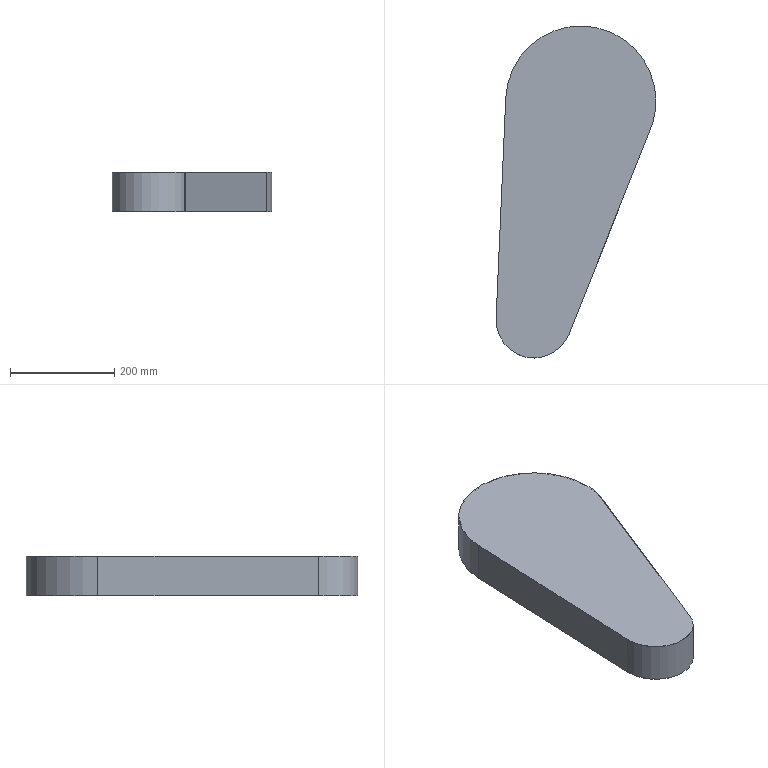Part | SolidWorks | features BaseBody 1 | 1 solid | 13 faces | box 306.5 x 636.5 x 76.6 mm | volume 401718 mm3 | plane 7 | cylinder 6 | commonest cylinder face diameters 141.8 x2 288 x2 145 x1 284.8 x1
STEP:
#1=CARTESIAN_POINT('',(350.539,286.374,-75.));
#2=VERTEX_POINT('',#1);
#3=CARTESIAN_POINT('',(360.722,339.564,-75.));
#4=VERTEX_POINT('',#3);
#5=CARTESIAN_POINT('',(216.722,339.564,-75.));
#6=DIRECTION('',(0.,0.,1.));
#7=DIRECTION('',(1.,0.,0.));
#8=AXIS2_PLACEMENT_3D('',#5,#6,#7);
#9=CIRCLE('',#8,144.);
#10=EDGE_CURVE('',#2,#4,#9,.T.);
#11=ORIENTED_EDGE('',*,*,#10,.T.);
#12=CARTESIAN_POINT('',(360.722,339.564,1.6));
#13=VERTEX_POINT('',#12);
#14=CARTESIAN_POINT('',(360.722,339.564,0.));
#15=DIRECTION('',(0.,0.,1.));
#16=VECTOR('',#15,1000.);
#17=LINE('',#14,#16);
#18=EDGE_CURVE('',#4,#13,#17,.T.);
#19=ORIENTED_EDGE('',*,*,#18,.T.);
#20=CARTESIAN_POINT('',(350.539,286.374,1.6));
#21=VERTEX_POINT('',#20);
#22=CARTESIAN_POINT('',(216.722,339.564,1.6));
#23=DIRECTION('',(0.,0.,1.));
#24=DIRECTION('',(1.,0.,0.));
#25=AXIS2_PLACEMENT_3D('',#22,#23,#24);
#26=CIRCLE('',#25,144.);
#27=EDGE_CURVE('',#21,#13,#26,.T.);
#28=ORIENTED_EDGE('',*,*,#27,.F.);
#29=CARTESIAN_POINT('',(350.539,286.374,0.));
#30=DIRECTION('',(0.,0.,-1.));
#31=VECTOR('',#30,1000.);
#32=LINE('',#29,#31);
#33=EDGE_CURVE('',#21,#2,#32,.T.);
#34=ORIENTED_EDGE('',*,*,#33,.T.);
#35=EDGE_LOOP('',(#11,#19,#28,#34));
#36=FACE_OUTER_BOUND('',#35,.T.);
#37=CARTESIAN_POINT('',(216.722,339.564,0.));
#38=DIRECTION('',(0.,0.,1.));
#39=DIRECTION('',(1.,0.,0.));
#40=AXIS2_PLACEMENT_3D('',#37,#38,#39);
#41=CYLINDRICAL_SURFACE('',#40,144.);
#42=ADVANCED_FACE('',(#36),#41,.T.);
#43=CARTESIAN_POINT('',(55.822,-80.436,0.));
#44=VERTEX_POINT('',#43);
#45=CARTESIAN_POINT('',(55.89,-77.328,0.));
#46=VERTEX_POINT('',#45);
#47=CARTESIAN_POINT('',(126.722,-80.436,0.));
#48=DIRECTION('',(0.,0.,-1.));
#49=DIRECTION('',(-1.,0.,0.));
#50=AXIS2_PLACEMENT_3D('',#47,#48,#49);
#51=CIRCLE('',#50,70.9);
#52=EDGE_CURVE('',#44,#46,#51,.T.);
#53=ORIENTED_EDGE('',*,*,#52,.F.);
#54=CARTESIAN_POINT('',(55.822,-80.436,-75.));
#55=VERTEX_POINT('',#54);
#56=CARTESIAN_POINT('',(55.822,-80.436,0.));
#57=DIRECTION('',(0.,0.,-1.));
#58=VECTOR('',#57,1000.);
#59=LINE('',#56,#58);
#60=EDGE_CURVE('',#44,#55,#59,.T.);
#61=ORIENTED_EDGE('',*,*,#60,.T.);
#62=CARTESIAN_POINT('',(55.89,-77.328,-75.));
#63=VERTEX_POINT('',#62);
#64=CARTESIAN_POINT('',(126.722,-80.436,-75.));
#65=DIRECTION('',(0.,0.,-1.));
#66=DIRECTION('',(-1.,0.,0.));
#67=AXIS2_PLACEMENT_3D('',#64,#65,#66);
#68=CIRCLE('',#67,70.9);
#69=EDGE_CURVE('',#55,#63,#68,.T.);
#70=ORIENTED_EDGE('',*,*,#69,.T.);
#71=CARTESIAN_POINT('',(55.89,-77.328,0.));
#72=DIRECTION('',(0.,0.,1.));
#73=VECTOR('',#72,1000.);
#74=LINE('',#71,#73);
#75=EDGE_CURVE('',#63,#46,#74,.T.);
#76=ORIENTED_EDGE('',*,*,#75,.T.);
#77=EDGE_LOOP('',(#53,#61,#70,#76));
#78=FACE_OUTER_BOUND('',#77,.T.);
#79=CARTESIAN_POINT('',(126.722,-80.436,0.));
#80=DIRECTION('',(0.,0.,-1.));
#81=DIRECTION('',(-1.,0.,0.));
#82=AXIS2_PLACEMENT_3D('',#79,#80,#81);
#83=CYLINDRICAL_SURFACE('',#82,70.9);
#84=ADVANCED_FACE('',(#78),#83,.F.);
#85=CARTESIAN_POINT('',(72.86,345.877,1.6));
#86=VERTEX_POINT('',#85);
#87=CARTESIAN_POINT('',(54.292,-77.258,1.6));
#88=VERTEX_POINT('',#87);
#89=CARTESIAN_POINT('',(72.86,345.877,1.6));
#90=DIRECTION('',(-0.04384,-0.999,0.));
#91=VECTOR('',#90,1000.);
#92=LINE('',#89,#91);
#93=EDGE_CURVE('',#86,#88,#92,.T.);
#94=ORIENTED_EDGE('',*,*,#93,.T.);
#95=CARTESIAN_POINT('',(194.095,-107.216,1.6));
#96=VERTEX_POINT('',#95);
#97=CARTESIAN_POINT('',(126.722,-80.436,1.6));
#98=DIRECTION('',(0.,0.,1.));
#99=DIRECTION('',(1.,0.,0.));
#100=AXIS2_PLACEMENT_3D('',#97,#98,#99);
#101=CIRCLE('',#100,72.5);
#102=EDGE_CURVE('',#88,#96,#101,.T.);
#103=ORIENTED_EDGE('',*,*,#102,.T.);
#104=CARTESIAN_POINT('',(194.095,-107.216,1.6));
#105=DIRECTION('',(0.3694,0.9293,0.));
#106=VECTOR('',#105,1000.);
#107=LINE('',#104,#106);
#108=EDGE_CURVE('',#96,#21,#107,.T.);
#109=ORIENTED_EDGE('',*,*,#108,.T.);
#110=ORIENTED_EDGE('',*,*,#27,.T.);
#111=CARTESIAN_POINT('',(216.722,339.564,1.6));
#112=DIRECTION('',(0.,0.,1.));
#113=DIRECTION('',(1.,0.,0.));
#114=AXIS2_PLACEMENT_3D('',#111,#112,#113);
#115=CIRCLE('',#114,144.);
#116=EDGE_CURVE('',#13,#86,#115,.T.);
#117=ORIENTED_EDGE('',*,*,#116,.T.);
#118=EDGE_LOOP('',(#94,#103,#109,#110,#117));
#119=FACE_OUTER_BOUND('',#118,.T.);
#120=CARTESIAN_POINT('',(181.806,176.624,1.6));
#121=DIRECTION('',(0.,0.,1.));
#122=DIRECTION('',(1.,0.,0.));
#123=AXIS2_PLACEMENT_3D('',#120,#121,#122);
#124=PLANE('',#123);
#125=ADVANCED_FACE('',(#119),#124,.T.);
#126=CARTESIAN_POINT('',(54.292,-77.258,-75.));
#127=VERTEX_POINT('',#126);
#128=CARTESIAN_POINT('',(194.095,-107.216,-75.));
#129=VERTEX_POINT('',#128);
#130=CARTESIAN_POINT('',(126.722,-80.436,-75.));
#131=DIRECTION('',(0.,0.,1.));
#132=DIRECTION('',(1.,0.,0.));
#133=AXIS2_PLACEMENT_3D('',#130,#131,#132);
#134=CIRCLE('',#133,72.5);
#135=EDGE_CURVE('',#127,#129,#134,.T.);
#136=ORIENTED_EDGE('',*,*,#135,.T.);
#137=CARTESIAN_POINT('',(194.095,-107.216,0.));
#138=DIRECTION('',(0.,0.,1.));
#139=VECTOR('',#138,1000.);
#140=LINE('',#137,#139);
#141=EDGE_CURVE('',#129,#96,#140,.T.);
#142=ORIENTED_EDGE('',*,*,#141,.T.);
#143=ORIENTED_EDGE('',*,*,#102,.F.);
#144=CARTESIAN_POINT('',(54.292,-77.258,0.));
#145=DIRECTION('',(0.,0.,-1.));
#146=VECTOR('',#145,1000.);
#147=LINE('',#144,#146);
#148=EDGE_CURVE('',#88,#127,#147,.T.);
#149=ORIENTED_EDGE('',*,*,#148,.T.);
#150=EDGE_LOOP('',(#136,#142,#143,#149));
#151=FACE_OUTER_BOUND('',#150,.T.);
#152=CARTESIAN_POINT('',(126.722,-80.436,0.));
#153=DIRECTION('',(0.,0.,1.));
#154=DIRECTION('',(1.,0.,0.));
#155=AXIS2_PLACEMENT_3D('',#152,#153,#154);
#156=CYLINDRICAL_SURFACE('',#155,72.5);
#157=ADVANCED_FACE('',(#151),#156,.T.);
#158=CARTESIAN_POINT('',(72.86,345.877,-75.));
#159=VERTEX_POINT('',#158);
#160=CARTESIAN_POINT('',(54.292,-77.258,-75.));
#161=DIRECTION('',(-0.04384,-0.999,0.));
#162=VECTOR('',#161,1000.);
#163=LINE('',#160,#162);
#164=EDGE_CURVE('',#159,#127,#163,.T.);
#165=ORIENTED_EDGE('',*,*,#164,.T.);
#166=ORIENTED_EDGE('',*,*,#148,.F.);
#167=ORIENTED_EDGE('',*,*,#93,.F.);
#168=CARTESIAN_POINT('',(72.86,345.877,0.));
#169=DIRECTION('',(0.,0.,-1.));
#170=VECTOR('',#169,1000.);
#171=LINE('',#168,#170);
#172=EDGE_CURVE('',#86,#159,#171,.T.);
#173=ORIENTED_EDGE('',*,*,#172,.T.);
#174=EDGE_LOOP('',(#165,#166,#167,#173));
#175=FACE_OUTER_BOUND('',#174,.T.);
#176=CARTESIAN_POINT('',(54.292,-77.258,0.));
#177=DIRECTION('',(-0.999,0.04384,0.));
#178=DIRECTION('',(-0.04384,-0.999,0.));
#179=AXIS2_PLACEMENT_3D('',#176,#177,#178);
#180=PLANE('',#179);
#181=ADVANCED_FACE('',(#175),#180,.T.);
#182=ORIENTED_EDGE('',*,*,#18,.F.);
#183=CARTESIAN_POINT('',(216.722,339.564,-75.));
#184=DIRECTION('',(0.,0.,1.));
#185=DIRECTION('',(1.,0.,0.));
#186=AXIS2_PLACEMENT_3D('',#183,#184,#185);
#187=CIRCLE('',#186,144.);
#188=EDGE_CURVE('',#4,#159,#187,.T.);
#189=ORIENTED_EDGE('',*,*,#188,.T.);
#190=ORIENTED_EDGE('',*,*,#172,.F.);
#191=ORIENTED_EDGE('',*,*,#116,.F.);
#192=EDGE_LOOP('',(#182,#189,#190,#191));
#193=FACE_OUTER_BOUND('',#192,.T.);
#194=CARTESIAN_POINT('',(216.722,339.564,0.));
#195=DIRECTION('',(0.,0.,1.));
#196=DIRECTION('',(1.,0.,0.));
#197=AXIS2_PLACEMENT_3D('',#194,#195,#196);
#198=CYLINDRICAL_SURFACE('',#197,144.);
#199=ADVANCED_FACE('',(#193),#198,.T.);
#200=CARTESIAN_POINT('',(350.539,286.374,-75.));
#201=DIRECTION('',(0.3694,0.9293,0.));
#202=VECTOR('',#201,1000.);
#203=LINE('',#200,#202);
#204=EDGE_CURVE('',#129,#2,#203,.T.);
#205=ORIENTED_EDGE('',*,*,#204,.T.);
#206=ORIENTED_EDGE('',*,*,#33,.F.);
#207=ORIENTED_EDGE('',*,*,#108,.F.);
#208=ORIENTED_EDGE('',*,*,#141,.F.);
#209=EDGE_LOOP('',(#205,#206,#207,#208));
#210=FACE_OUTER_BOUND('',#209,.T.);
#211=CARTESIAN_POINT('',(350.539,286.374,0.));
#212=DIRECTION('',(0.9293,-0.3694,0.));
#213=DIRECTION('',(0.3694,0.9293,0.));
#214=AXIS2_PLACEMENT_3D('',#211,#212,#213);
#215=PLANE('',#214);
#216=ADVANCED_FACE('',(#210),#215,.T.);
#217=CARTESIAN_POINT('',(192.608,-106.625,-75.));
#218=VERTEX_POINT('',#217);
#219=CARTESIAN_POINT('',(126.722,-80.436,-75.));
#220=DIRECTION('',(0.,0.,-1.));
#221=DIRECTION('',(-1.,0.,0.));
#222=AXIS2_PLACEMENT_3D('',#219,#220,#221);
#223=CIRCLE('',#222,70.9);
#224=EDGE_CURVE('',#218,#55,#223,.T.);
#225=ORIENTED_EDGE('',*,*,#224,.F.);
#226=CARTESIAN_POINT('',(349.052,286.965,-75.));
#227=VERTEX_POINT('',#226);
#228=CARTESIAN_POINT('',(349.052,286.965,-75.));
#229=DIRECTION('',(-0.3694,-0.9293,0.));
#230=VECTOR('',#229,1000.);
#231=LINE('',#228,#230);
#232=EDGE_CURVE('',#227,#218,#231,.T.);
#233=ORIENTED_EDGE('',*,*,#232,.F.);
#234=CARTESIAN_POINT('',(74.459,345.807,-75.));
#235=VERTEX_POINT('',#234);
#236=CARTESIAN_POINT('',(216.722,339.564,-75.));
#237=DIRECTION('',(0.,0.,-1.));
#238=DIRECTION('',(-1.,0.,0.));
#239=AXIS2_PLACEMENT_3D('',#236,#237,#238);
#240=CIRCLE('',#239,142.4);
#241=EDGE_CURVE('',#235,#227,#240,.T.);
#242=ORIENTED_EDGE('',*,*,#241,.F.);
#243=CARTESIAN_POINT('',(55.89,-77.328,-75.));
#244=DIRECTION('',(0.04384,0.999,0.));
#245=VECTOR('',#244,1000.);
#246=LINE('',#243,#245);
#247=EDGE_CURVE('',#63,#235,#246,.T.);
#248=ORIENTED_EDGE('',*,*,#247,.F.);
#249=ORIENTED_EDGE('',*,*,#69,.F.);
#250=EDGE_LOOP('',(#225,#233,#242,#248,#249));
#251=FACE_BOUND('',#250,.T.);
#252=ORIENTED_EDGE('',*,*,#10,.F.);
#253=ORIENTED_EDGE('',*,*,#204,.F.);
#254=ORIENTED_EDGE('',*,*,#135,.F.);
#255=ORIENTED_EDGE('',*,*,#164,.F.);
#256=ORIENTED_EDGE('',*,*,#188,.F.);
#257=EDGE_LOOP('',(#252,#253,#254,#255,#256));
#258=FACE_OUTER_BOUND('',#257,.T.);
#259=CARTESIAN_POINT('',(181.806,176.624,-75.));
#260=DIRECTION('',(0.,0.,1.));
#261=DIRECTION('',(1.,0.,0.));
#262=AXIS2_PLACEMENT_3D('',#259,#260,#261);
#263=PLANE('',#262);
#264=ADVANCED_FACE('',(#251,#258),#263,.F.);
#265=CARTESIAN_POINT('',(74.459,345.807,0.));
#266=VERTEX_POINT('',#265);
#267=CARTESIAN_POINT('',(74.459,345.807,0.));
#268=DIRECTION('',(0.,0.,-1.));
#269=VECTOR('',#268,1000.);
#270=LINE('',#267,#269);
#271=EDGE_CURVE('',#266,#235,#270,.T.);
#272=ORIENTED_EDGE('',*,*,#271,.F.);
#273=CARTESIAN_POINT('',(74.459,345.807,0.));
#274=DIRECTION('',(0.04384,0.999,0.));
#275=VECTOR('',#274,1000.);
#276=LINE('',#273,#275);
#277=EDGE_CURVE('',#46,#266,#276,.T.);
#278=ORIENTED_EDGE('',*,*,#277,.F.);
#279=ORIENTED_EDGE('',*,*,#75,.F.);
#280=ORIENTED_EDGE('',*,*,#247,.T.);
#281=EDGE_LOOP('',(#272,#278,#279,#280));
#282=FACE_OUTER_BOUND('',#281,.T.);
#283=CARTESIAN_POINT('',(74.459,345.807,0.));
#284=DIRECTION('',(-0.999,0.04384,0.));
#285=DIRECTION('',(-0.04384,-0.999,0.));
#286=AXIS2_PLACEMENT_3D('',#283,#284,#285);
#287=PLANE('',#286);
#288=ADVANCED_FACE('',(#282),#287,.F.);
#289=ORIENTED_EDGE('',*,*,#60,.F.);
#290=CARTESIAN_POINT('',(192.608,-106.625,0.));
#291=VERTEX_POINT('',#290);
#292=CARTESIAN_POINT('',(126.722,-80.436,0.));
#293=DIRECTION('',(0.,0.,-1.));
#294=DIRECTION('',(-1.,0.,0.));
#295=AXIS2_PLACEMENT_3D('',#292,#293,#294);
#296=CIRCLE('',#295,70.9);
#297=EDGE_CURVE('',#291,#44,#296,.T.);
#298=ORIENTED_EDGE('',*,*,#297,.F.);
#299=CARTESIAN_POINT('',(192.608,-106.625,0.));
#300=DIRECTION('',(0.,0.,1.));
#301=VECTOR('',#300,1000.);
#302=LINE('',#299,#301);
#303=EDGE_CURVE('',#218,#291,#302,.T.);
#304=ORIENTED_EDGE('',*,*,#303,.F.);
#305=ORIENTED_EDGE('',*,*,#224,.T.);
#306=EDGE_LOOP('',(#289,#298,#304,#305));
#307=FACE_OUTER_BOUND('',#306,.T.);
#308=CARTESIAN_POINT('',(126.722,-80.436,0.));
#309=DIRECTION('',(0.,0.,-1.));
#310=DIRECTION('',(-1.,0.,0.));
#311=AXIS2_PLACEMENT_3D('',#308,#309,#310);
#312=CYLINDRICAL_SURFACE('',#311,70.9);
#313=ADVANCED_FACE('',(#307),#312,.F.);
#314=ORIENTED_EDGE('',*,*,#303,.T.);
#315=CARTESIAN_POINT('',(349.052,286.965,0.));
#316=VERTEX_POINT('',#315);
#317=CARTESIAN_POINT('',(192.608,-106.625,0.));
#318=DIRECTION('',(-0.3694,-0.9293,0.));
#319=VECTOR('',#318,1000.);
#320=LINE('',#317,#319);
#321=EDGE_CURVE('',#316,#291,#320,.T.);
#322=ORIENTED_EDGE('',*,*,#321,.F.);
#323=CARTESIAN_POINT('',(349.052,286.965,0.));
#324=DIRECTION('',(0.,0.,1.));
#325=VECTOR('',#324,1000.);
#326=LINE('',#323,#325);
#327=EDGE_CURVE('',#227,#316,#326,.T.);
#328=ORIENTED_EDGE('',*,*,#327,.F.);
#329=ORIENTED_EDGE('',*,*,#232,.T.);
#330=EDGE_LOOP('',(#314,#322,#328,#329));
#331=FACE_OUTER_BOUND('',#330,.T.);
#332=CARTESIAN_POINT('',(192.608,-106.625,0.));
#333=DIRECTION('',(0.9293,-0.3694,0.));
#334=DIRECTION('',(0.3694,0.9293,0.));
#335=AXIS2_PLACEMENT_3D('',#332,#333,#334);
#336=PLANE('',#335);
#337=ADVANCED_FACE('',(#331),#336,.F.);
#338=ORIENTED_EDGE('',*,*,#327,.T.);
#339=CARTESIAN_POINT('',(216.722,339.564,0.));
#340=DIRECTION('',(0.,0.,-1.));
#341=DIRECTION('',(-1.,0.,0.));
#342=AXIS2_PLACEMENT_3D('',#339,#340,#341);
#343=CIRCLE('',#342,142.4);
#344=EDGE_CURVE('',#266,#316,#343,.T.);
#345=ORIENTED_EDGE('',*,*,#344,.F.);
#346=ORIENTED_EDGE('',*,*,#271,.T.);
#347=ORIENTED_EDGE('',*,*,#241,.T.);
#348=EDGE_LOOP('',(#338,#345,#346,#347));
#349=FACE_OUTER_BOUND('',#348,.T.);
#350=CARTESIAN_POINT('',(216.722,339.564,0.));
#351=DIRECTION('',(0.,0.,-1.));
#352=DIRECTION('',(-1.,0.,0.));
#353=AXIS2_PLACEMENT_3D('',#350,#351,#352);
#354=CYLINDRICAL_SURFACE('',#353,142.4);
#355=ADVANCED_FACE('',(#349),#354,.F.);
#356=ORIENTED_EDGE('',*,*,#344,.T.);
#357=ORIENTED_EDGE('',*,*,#321,.T.);
#358=ORIENTED_EDGE('',*,*,#297,.T.);
#359=ORIENTED_EDGE('',*,*,#52,.T.);
#360=ORIENTED_EDGE('',*,*,#277,.T.);
#361=EDGE_LOOP('',(#356,#357,#358,#359,#360));
#362=FACE_OUTER_BOUND('',#361,.T.);
#363=CARTESIAN_POINT('',(181.806,176.624,0.));
#364=DIRECTION('',(0.,0.,1.));
#365=DIRECTION('',(1.,0.,0.));
#366=AXIS2_PLACEMENT_3D('',#363,#364,#365);
#367=PLANE('',#366);
#368=ADVANCED_FACE('',(#362),#367,.F.);
#369=CLOSED_SHELL('',(#42,#84,#125,#157,#181,#199,#216,#264,#288,#313,#337,#355,#368));
#370=MANIFOLD_SOLID_BREP('',#369);
#371=CARTESIAN_POINT('',(0.,0.,0.));
#372=DIRECTION('',(0.,0.,1.));
#373=DIRECTION('',(1.,0.,0.));
#374=AXIS2_PLACEMENT_3D('',#371,#372,#373);
#375=(LENGTH_UNIT()NAMED_UNIT(*)SI_UNIT(.MILLI.,.METRE.));
#376=UNCERTAINTY_MEASURE_WITH_UNIT(LENGTH_MEASURE(0.00001),#375,'','');
#377=(NAMED_UNIT(*)PLANE_ANGLE_UNIT()SI_UNIT($,.RADIAN.));
#378=(NAMED_UNIT(*)SI_UNIT($,.STERADIAN.)SOLID_ANGLE_UNIT());
#379=(GEOMETRIC_REPRESENTATION_CONTEXT(3)GLOBAL_UNCERTAINTY_ASSIGNED_CONTEXT((#376))GLOBAL_UNIT_ASSIGNED_CONTEXT((#375,#377,#378))REPRESENTATION_CONTEXT('',''));
#380=ADVANCED_BREP_SHAPE_REPRESENTATION('',(#370,#374),#379);